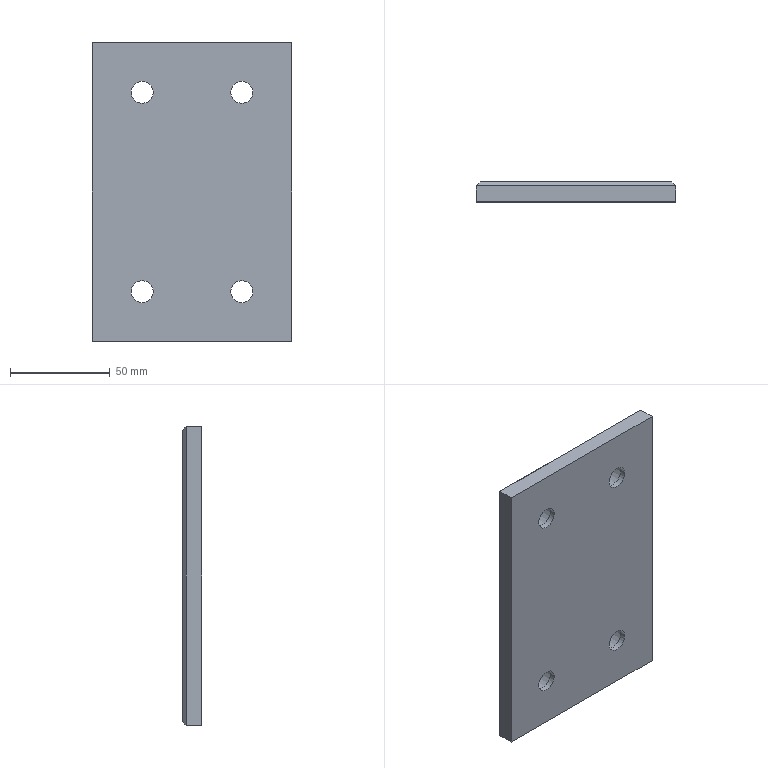Part | NX | features solid 2 | 1 solid | 22 faces | box 100 x 10 x 150 mm | volume 140961 mm3 | plane 14 | cylinder 8 | commonest cylinder face diameters 11 x4 17.5 x4
STEP:
#1=CARTESIAN_POINT('',(45.,37.,109.));
#2=VERTEX_POINT('',#1);
#3=CARTESIAN_POINT('',(45.,45.,109.));
#4=VERTEX_POINT('',#3);
#5=CARTESIAN_POINT('',(45.,37.,109.));
#6=DIRECTION('',(0.,1.,0.));
#7=VECTOR('',#6,1000.);
#8=LINE('',#5,#7);
#9=EDGE_CURVE('',#2,#4,#8,.T.);
#10=ORIENTED_EDGE('',*,*,#9,.T.);
#11=CARTESIAN_POINT('',(45.,45.,259.));
#12=VERTEX_POINT('',#11);
#13=CARTESIAN_POINT('',(45.,45.,259.));
#14=DIRECTION('',(0.,0.,1.));
#15=VECTOR('',#14,1000.);
#16=LINE('',#13,#15);
#17=EDGE_CURVE('',#4,#12,#16,.T.);
#18=ORIENTED_EDGE('',*,*,#17,.T.);
#19=CARTESIAN_POINT('',(45.,37.,259.));
#20=VERTEX_POINT('',#19);
#21=CARTESIAN_POINT('',(45.,37.,259.));
#22=DIRECTION('',(0.,1.,0.));
#23=VECTOR('',#22,1000.);
#24=LINE('',#21,#23);
#25=EDGE_CURVE('',#20,#12,#24,.T.);
#26=ORIENTED_EDGE('',*,*,#25,.F.);
#27=CARTESIAN_POINT('',(45.,37.,259.));
#28=DIRECTION('',(0.,0.,-1.));
#29=VECTOR('',#28,1000.);
#30=LINE('',#27,#29);
#31=EDGE_CURVE('',#2,#20,#30,.F.);
#32=ORIENTED_EDGE('',*,*,#31,.F.);
#33=EDGE_LOOP('',(#10,#18,#26,#32));
#34=FACE_BOUND('',#33,.T.);
#35=CARTESIAN_POINT('',(45.,37.,259.));
#36=DIRECTION('',(-1.,0.,0.));
#37=DIRECTION('',(0.,0.,1.));
#38=AXIS2_PLACEMENT_3D('',#35,#36,#37);
#39=PLANE('',#38);
#40=ADVANCED_FACE('',(#34),#39,.F.);
#41=CARTESIAN_POINT('',(-55.,37.,109.));
#42=VERTEX_POINT('',#41);
#43=CARTESIAN_POINT('',(-55.,45.,109.));
#44=VERTEX_POINT('',#43);
#45=CARTESIAN_POINT('',(-55.,37.,109.));
#46=DIRECTION('',(0.,1.,0.));
#47=VECTOR('',#46,1000.);
#48=LINE('',#45,#47);
#49=EDGE_CURVE('',#42,#44,#48,.T.);
#50=ORIENTED_EDGE('',*,*,#49,.T.);
#51=CARTESIAN_POINT('',(70.,45.,109.));
#52=DIRECTION('',(1.,0.,0.));
#53=VECTOR('',#52,1000.);
#54=LINE('',#51,#53);
#55=EDGE_CURVE('',#44,#4,#54,.T.);
#56=ORIENTED_EDGE('',*,*,#55,.T.);
#57=ORIENTED_EDGE('',*,*,#9,.F.);
#58=CARTESIAN_POINT('',(70.,37.,109.));
#59=DIRECTION('',(-1.,0.,0.));
#60=VECTOR('',#59,1000.);
#61=LINE('',#58,#60);
#62=EDGE_CURVE('',#2,#42,#61,.T.);
#63=ORIENTED_EDGE('',*,*,#62,.T.);
#64=EDGE_LOOP('',(#50,#56,#57,#63));
#65=FACE_BOUND('',#64,.T.);
#66=CARTESIAN_POINT('',(70.,37.,109.));
#67=DIRECTION('',(0.,0.,-1.));
#68=DIRECTION('',(-1.,0.,0.));
#69=AXIS2_PLACEMENT_3D('',#66,#67,#68);
#70=PLANE('',#69);
#71=ADVANCED_FACE('',(#65),#70,.T.);
#72=CARTESIAN_POINT('',(-55.,37.,259.));
#73=VERTEX_POINT('',#72);
#74=CARTESIAN_POINT('',(-55.,45.,259.));
#75=VERTEX_POINT('',#74);
#76=CARTESIAN_POINT('',(-55.,37.,259.));
#77=DIRECTION('',(0.,1.,0.));
#78=VECTOR('',#77,1000.);
#79=LINE('',#76,#78);
#80=EDGE_CURVE('',#73,#75,#79,.T.);
#81=ORIENTED_EDGE('',*,*,#80,.T.);
#82=CARTESIAN_POINT('',(-55.,45.,259.));
#83=DIRECTION('',(0.,0.,-1.));
#84=VECTOR('',#83,1000.);
#85=LINE('',#82,#84);
#86=EDGE_CURVE('',#75,#44,#85,.T.);
#87=ORIENTED_EDGE('',*,*,#86,.T.);
#88=ORIENTED_EDGE('',*,*,#49,.F.);
#89=CARTESIAN_POINT('',(-55.,37.,259.));
#90=DIRECTION('',(0.,0.,1.));
#91=VECTOR('',#90,1000.);
#92=LINE('',#89,#91);
#93=EDGE_CURVE('',#73,#42,#92,.F.);
#94=ORIENTED_EDGE('',*,*,#93,.F.);
#95=EDGE_LOOP('',(#81,#87,#88,#94));
#96=FACE_BOUND('',#95,.T.);
#97=CARTESIAN_POINT('',(-55.,37.,259.));
#98=DIRECTION('',(1.,0.,0.));
#99=DIRECTION('',(0.,0.,-1.));
#100=AXIS2_PLACEMENT_3D('',#97,#98,#99);
#101=PLANE('',#100);
#102=ADVANCED_FACE('',(#96),#101,.F.);
#103=ORIENTED_EDGE('',*,*,#25,.T.);
#104=CARTESIAN_POINT('',(-80.,45.,259.));
#105=DIRECTION('',(-1.,0.,0.));
#106=VECTOR('',#105,1000.);
#107=LINE('',#104,#106);
#108=EDGE_CURVE('',#12,#75,#107,.T.);
#109=ORIENTED_EDGE('',*,*,#108,.T.);
#110=ORIENTED_EDGE('',*,*,#80,.F.);
#111=CARTESIAN_POINT('',(-80.,37.,259.));
#112=DIRECTION('',(1.,0.,0.));
#113=VECTOR('',#112,1000.);
#114=LINE('',#111,#113);
#115=EDGE_CURVE('',#20,#73,#114,.F.);
#116=ORIENTED_EDGE('',*,*,#115,.F.);
#117=EDGE_LOOP('',(#103,#109,#110,#116));
#118=FACE_BOUND('',#117,.T.);
#119=CARTESIAN_POINT('',(-80.,37.,259.));
#120=DIRECTION('',(0.,0.,-1.));
#121=DIRECTION('',(-1.,0.,0.));
#122=AXIS2_PLACEMENT_3D('',#119,#120,#121);
#123=PLANE('',#122);
#124=ADVANCED_FACE('',(#118),#123,.F.);
#125=CARTESIAN_POINT('',(-30.,37.,228.5));
#126=VERTEX_POINT('',#125);
#127=CARTESIAN_POINT('',(-30.,37.,234.));
#128=DIRECTION('',(0.,-1.,0.));
#129=DIRECTION('',(0.,0.,-1.));
#130=AXIS2_PLACEMENT_3D('',#127,#128,#129);
#131=CIRCLE('',#130,5.5);
#132=EDGE_CURVE('',#126,#126,#131,.T.);
#133=ORIENTED_EDGE('',*,*,#132,.F.);
#134=EDGE_LOOP('',(#133));
#135=FACE_BOUND('',#134,.T.);
#136=CARTESIAN_POINT('',(20.,37.,228.5));
#137=VERTEX_POINT('',#136);
#138=CARTESIAN_POINT('',(20.,37.,234.));
#139=DIRECTION('',(0.,-1.,0.));
#140=DIRECTION('',(0.,0.,-1.));
#141=AXIS2_PLACEMENT_3D('',#138,#139,#140);
#142=CIRCLE('',#141,5.5);
#143=EDGE_CURVE('',#137,#137,#142,.T.);
#144=ORIENTED_EDGE('',*,*,#143,.F.);
#145=EDGE_LOOP('',(#144));
#146=FACE_BOUND('',#145,.T.);
#147=CARTESIAN_POINT('',(-30.,37.,128.5));
#148=VERTEX_POINT('',#147);
#149=CARTESIAN_POINT('',(-30.,37.,134.));
#150=DIRECTION('',(0.,-1.,0.));
#151=DIRECTION('',(0.,0.,-1.));
#152=AXIS2_PLACEMENT_3D('',#149,#150,#151);
#153=CIRCLE('',#152,5.5);
#154=EDGE_CURVE('',#148,#148,#153,.T.);
#155=ORIENTED_EDGE('',*,*,#154,.F.);
#156=EDGE_LOOP('',(#155));
#157=FACE_BOUND('',#156,.T.);
#158=CARTESIAN_POINT('',(20.,37.,128.5));
#159=VERTEX_POINT('',#158);
#160=CARTESIAN_POINT('',(20.,37.,134.));
#161=DIRECTION('',(0.,-1.,0.));
#162=DIRECTION('',(0.,0.,-1.));
#163=AXIS2_PLACEMENT_3D('',#160,#161,#162);
#164=CIRCLE('',#163,5.5);
#165=EDGE_CURVE('',#159,#159,#164,.T.);
#166=ORIENTED_EDGE('',*,*,#165,.F.);
#167=EDGE_LOOP('',(#166));
#168=FACE_BOUND('',#167,.T.);
#169=ORIENTED_EDGE('',*,*,#31,.T.);
#170=ORIENTED_EDGE('',*,*,#115,.T.);
#171=ORIENTED_EDGE('',*,*,#93,.T.);
#172=ORIENTED_EDGE('',*,*,#62,.F.);
#173=EDGE_LOOP('',(#169,#170,#171,#172));
#174=FACE_BOUND('',#173,.T.);
#175=CARTESIAN_POINT('',(70.,37.,259.));
#176=DIRECTION('',(0.,-1.,0.));
#177=DIRECTION('',(0.,0.,1.));
#178=AXIS2_PLACEMENT_3D('',#175,#176,#177);
#179=PLANE('',#178);
#180=ADVANCED_FACE('',(#135,#146,#157,#168,#174),#179,.T.);
#181=CARTESIAN_POINT('',(-30.,47.,225.25));
#182=VERTEX_POINT('',#181);
#183=CARTESIAN_POINT('',(-30.,47.,234.));
#184=DIRECTION('',(0.,-1.,0.));
#185=DIRECTION('',(0.,0.,-1.));
#186=AXIS2_PLACEMENT_3D('',#183,#184,#185);
#187=CIRCLE('',#186,8.75);
#188=EDGE_CURVE('',#182,#182,#187,.T.);
#189=ORIENTED_EDGE('',*,*,#188,.T.);
#190=EDGE_LOOP('',(#189));
#191=FACE_BOUND('',#190,.T.);
#192=CARTESIAN_POINT('',(20.,47.,225.25));
#193=VERTEX_POINT('',#192);
#194=CARTESIAN_POINT('',(20.,47.,234.));
#195=DIRECTION('',(0.,-1.,0.));
#196=DIRECTION('',(0.,0.,-1.));
#197=AXIS2_PLACEMENT_3D('',#194,#195,#196);
#198=CIRCLE('',#197,8.75);
#199=EDGE_CURVE('',#193,#193,#198,.T.);
#200=ORIENTED_EDGE('',*,*,#199,.T.);
#201=EDGE_LOOP('',(#200));
#202=FACE_BOUND('',#201,.T.);
#203=CARTESIAN_POINT('',(-30.,47.,125.25));
#204=VERTEX_POINT('',#203);
#205=CARTESIAN_POINT('',(-30.,47.,134.));
#206=DIRECTION('',(0.,-1.,0.));
#207=DIRECTION('',(0.,0.,-1.));
#208=AXIS2_PLACEMENT_3D('',#205,#206,#207);
#209=CIRCLE('',#208,8.75);
#210=EDGE_CURVE('',#204,#204,#209,.T.);
#211=ORIENTED_EDGE('',*,*,#210,.T.);
#212=EDGE_LOOP('',(#211));
#213=FACE_BOUND('',#212,.T.);
#214=CARTESIAN_POINT('',(20.,47.,125.25));
#215=VERTEX_POINT('',#214);
#216=CARTESIAN_POINT('',(20.,47.,134.));
#217=DIRECTION('',(0.,-1.,0.));
#218=DIRECTION('',(0.,0.,-1.));
#219=AXIS2_PLACEMENT_3D('',#216,#217,#218);
#220=CIRCLE('',#219,8.75);
#221=EDGE_CURVE('',#215,#215,#220,.T.);
#222=ORIENTED_EDGE('',*,*,#221,.T.);
#223=EDGE_LOOP('',(#222));
#224=FACE_BOUND('',#223,.T.);
#225=CARTESIAN_POINT('',(43.,47.,111.));
#226=VERTEX_POINT('',#225);
#227=CARTESIAN_POINT('',(-53.,47.,111.));
#228=VERTEX_POINT('',#227);
#229=CARTESIAN_POINT('',(-80.,47.,111.));
#230=DIRECTION('',(-1.,0.,0.));
#231=VECTOR('',#230,1000.);
#232=LINE('',#229,#231);
#233=EDGE_CURVE('',#226,#228,#232,.T.);
#234=ORIENTED_EDGE('',*,*,#233,.T.);
#235=CARTESIAN_POINT('',(-53.,47.,257.));
#236=VERTEX_POINT('',#235);
#237=CARTESIAN_POINT('',(-53.,47.,259.));
#238=DIRECTION('',(0.,0.,1.));
#239=VECTOR('',#238,1000.);
#240=LINE('',#237,#239);
#241=EDGE_CURVE('',#228,#236,#240,.T.);
#242=ORIENTED_EDGE('',*,*,#241,.T.);
#243=CARTESIAN_POINT('',(43.,47.,257.));
#244=VERTEX_POINT('',#243);
#245=CARTESIAN_POINT('',(70.,47.,257.));
#246=DIRECTION('',(1.,0.,0.));
#247=VECTOR('',#246,1000.);
#248=LINE('',#245,#247);
#249=EDGE_CURVE('',#236,#244,#248,.T.);
#250=ORIENTED_EDGE('',*,*,#249,.T.);
#251=CARTESIAN_POINT('',(43.,47.,259.));
#252=DIRECTION('',(0.,0.,-1.));
#253=VECTOR('',#252,1000.);
#254=LINE('',#251,#253);
#255=EDGE_CURVE('',#244,#226,#254,.T.);
#256=ORIENTED_EDGE('',*,*,#255,.T.);
#257=EDGE_LOOP('',(#234,#242,#250,#256));
#258=FACE_BOUND('',#257,.T.);
#259=CARTESIAN_POINT('',(70.,47.,259.));
#260=DIRECTION('',(0.,-1.,0.));
#261=DIRECTION('',(0.,0.,1.));
#262=AXIS2_PLACEMENT_3D('',#259,#260,#261);
#263=PLANE('',#262);
#264=ADVANCED_FACE('',(#191,#202,#213,#224,#258),#263,.F.);
#265=CARTESIAN_POINT('',(43.667,46.333,110.333));
#266=DIRECTION('',(-0.5774,0.5774,0.5774));
#267=VECTOR('',#266,1000.);
#268=LINE('',#265,#267);
#269=EDGE_CURVE('',#226,#4,#268,.F.);
#270=ORIENTED_EDGE('',*,*,#269,.F.);
#271=ORIENTED_EDGE('',*,*,#255,.F.);
#272=CARTESIAN_POINT('',(45.,45.,259.));
#273=DIRECTION('',(0.5774,-0.5774,0.5774));
#274=VECTOR('',#273,1000.);
#275=LINE('',#272,#274);
#276=EDGE_CURVE('',#12,#244,#275,.F.);
#277=ORIENTED_EDGE('',*,*,#276,.F.);
#278=ORIENTED_EDGE('',*,*,#17,.F.);
#279=EDGE_LOOP('',(#270,#271,#277,#278));
#280=FACE_BOUND('',#279,.T.);
#281=CARTESIAN_POINT('',(45.,45.,259.));
#282=DIRECTION('',(-0.7071,-0.7071,0.));
#283=DIRECTION('',(0.7071,-0.7071,0.));
#284=AXIS2_PLACEMENT_3D('',#281,#282,#283);
#285=PLANE('',#284);
#286=ADVANCED_FACE('',(#280),#285,.F.);
#287=ORIENTED_EDGE('',*,*,#276,.T.);
#288=ORIENTED_EDGE('',*,*,#249,.F.);
#289=CARTESIAN_POINT('',(-55.,45.,259.));
#290=DIRECTION('',(-0.5774,-0.5774,0.5774));
#291=VECTOR('',#290,1000.);
#292=LINE('',#289,#291);
#293=EDGE_CURVE('',#75,#236,#292,.F.);
#294=ORIENTED_EDGE('',*,*,#293,.F.);
#295=ORIENTED_EDGE('',*,*,#108,.F.);
#296=EDGE_LOOP('',(#287,#288,#294,#295));
#297=FACE_BOUND('',#296,.T.);
#298=CARTESIAN_POINT('',(-80.,45.,259.));
#299=DIRECTION('',(0.,-0.7071,-0.7071));
#300=DIRECTION('',(0.,0.7071,-0.7071));
#301=AXIS2_PLACEMENT_3D('',#298,#299,#300);
#302=PLANE('',#301);
#303=ADVANCED_FACE('',(#297),#302,.F.);
#304=ORIENTED_EDGE('',*,*,#269,.T.);
#305=ORIENTED_EDGE('',*,*,#55,.F.);
#306=CARTESIAN_POINT('',(-3.667,96.333,160.333));
#307=DIRECTION('',(-0.5774,-0.5774,-0.5774));
#308=VECTOR('',#307,1000.);
#309=LINE('',#306,#308);
#310=EDGE_CURVE('',#228,#44,#309,.T.);
#311=ORIENTED_EDGE('',*,*,#310,.F.);
#312=ORIENTED_EDGE('',*,*,#233,.F.);
#313=EDGE_LOOP('',(#304,#305,#311,#312));
#314=FACE_BOUND('',#313,.T.);
#315=CARTESIAN_POINT('',(70.,47.,111.));
#316=DIRECTION('',(0.,0.7071,-0.7071));
#317=DIRECTION('',(0.,0.7071,0.7071));
#318=AXIS2_PLACEMENT_3D('',#315,#316,#317);
#319=PLANE('',#318);
#320=ADVANCED_FACE('',(#314),#319,.T.);
#321=ORIENTED_EDGE('',*,*,#293,.T.);
#322=ORIENTED_EDGE('',*,*,#241,.F.);
#323=ORIENTED_EDGE('',*,*,#310,.T.);
#324=ORIENTED_EDGE('',*,*,#86,.F.);
#325=EDGE_LOOP('',(#321,#322,#323,#324));
#326=FACE_BOUND('',#325,.T.);
#327=CARTESIAN_POINT('',(-55.,45.,259.));
#328=DIRECTION('',(0.7071,-0.7071,0.));
#329=DIRECTION('',(0.7071,0.7071,0.));
#330=AXIS2_PLACEMENT_3D('',#327,#328,#329);
#331=PLANE('',#330);
#332=ADVANCED_FACE('',(#326),#331,.F.);
#333=ORIENTED_EDGE('',*,*,#165,.T.);
#334=EDGE_LOOP('',(#333));
#335=FACE_BOUND('',#334,.T.);
#336=CARTESIAN_POINT('',(20.,39.7,128.5));
#337=VERTEX_POINT('',#336);
#338=CARTESIAN_POINT('',(20.,39.7,134.));
#339=DIRECTION('',(0.,-1.,0.));
#340=DIRECTION('',(0.,0.,-1.));
#341=AXIS2_PLACEMENT_3D('',#338,#339,#340);
#342=CIRCLE('',#341,5.5);
#343=EDGE_CURVE('',#337,#337,#342,.T.);
#344=ORIENTED_EDGE('',*,*,#343,.F.);
#345=EDGE_LOOP('',(#344));
#346=FACE_BOUND('',#345,.T.);
#347=CARTESIAN_POINT('',(20.,-3.,134.));
#348=DIRECTION('',(0.,-1.,0.));
#349=DIRECTION('',(0.,0.,-1.));
#350=AXIS2_PLACEMENT_3D('',#347,#348,#349);
#351=CYLINDRICAL_SURFACE('',#350,5.5);
#352=ADVANCED_FACE('',(#335,#346),#351,.F.);
#353=ORIENTED_EDGE('',*,*,#343,.T.);
#354=EDGE_LOOP('',(#353));
#355=FACE_BOUND('',#354,.T.);
#356=CARTESIAN_POINT('',(20.,39.7,125.25));
#357=VERTEX_POINT('',#356);
#358=CARTESIAN_POINT('',(20.,39.7,134.));
#359=DIRECTION('',(0.,-1.,0.));
#360=DIRECTION('',(0.,0.,-1.));
#361=AXIS2_PLACEMENT_3D('',#358,#359,#360);
#362=CIRCLE('',#361,8.75);
#363=EDGE_CURVE('',#357,#357,#362,.T.);
#364=ORIENTED_EDGE('',*,*,#363,.F.);
#365=EDGE_LOOP('',(#364));
#366=FACE_BOUND('',#365,.T.);
#367=CARTESIAN_POINT('',(45.,39.7,134.));
#368=DIRECTION('',(0.,-1.,0.));
#369=DIRECTION('',(0.,0.,-1.));
#370=AXIS2_PLACEMENT_3D('',#367,#368,#369);
#371=PLANE('',#370);
#372=ADVANCED_FACE('',(#355,#366),#371,.F.);
#373=ORIENTED_EDGE('',*,*,#363,.T.);
#374=EDGE_LOOP('',(#373));
#375=FACE_BOUND('',#374,.T.);
#376=ORIENTED_EDGE('',*,*,#221,.F.);
#377=EDGE_LOOP('',(#376));
#378=FACE_BOUND('',#377,.T.);
#379=CARTESIAN_POINT('',(20.,47.,134.));
#380=DIRECTION('',(0.,-1.,0.));
#381=DIRECTION('',(0.,0.,-1.));
#382=AXIS2_PLACEMENT_3D('',#379,#380,#381);
#383=CYLINDRICAL_SURFACE('',#382,8.75);
#384=ADVANCED_FACE('',(#375,#378),#383,.F.);
#385=ORIENTED_EDGE('',*,*,#154,.T.);
#386=EDGE_LOOP('',(#385));
#387=FACE_BOUND('',#386,.T.);
#388=CARTESIAN_POINT('',(-30.,39.7,128.5));
#389=VERTEX_POINT('',#388);
#390=CARTESIAN_POINT('',(-30.,39.7,134.));
#391=DIRECTION('',(0.,-1.,0.));
#392=DIRECTION('',(0.,0.,-1.));
#393=AXIS2_PLACEMENT_3D('',#390,#391,#392);
#394=CIRCLE('',#393,5.5);
#395=EDGE_CURVE('',#389,#389,#394,.T.);
#396=ORIENTED_EDGE('',*,*,#395,.F.);
#397=EDGE_LOOP('',(#396));
#398=FACE_BOUND('',#397,.T.);
#399=CARTESIAN_POINT('',(-30.,-3.,134.));
#400=DIRECTION('',(0.,-1.,0.));
#401=DIRECTION('',(0.,0.,-1.));
#402=AXIS2_PLACEMENT_3D('',#399,#400,#401);
#403=CYLINDRICAL_SURFACE('',#402,5.5);
#404=ADVANCED_FACE('',(#387,#398),#403,.F.);
#405=ORIENTED_EDGE('',*,*,#395,.T.);
#406=EDGE_LOOP('',(#405));
#407=FACE_BOUND('',#406,.T.);
#408=CARTESIAN_POINT('',(-30.,39.7,125.25));
#409=VERTEX_POINT('',#408);
#410=CARTESIAN_POINT('',(-30.,39.7,134.));
#411=DIRECTION('',(0.,-1.,0.));
#412=DIRECTION('',(0.,0.,-1.));
#413=AXIS2_PLACEMENT_3D('',#410,#411,#412);
#414=CIRCLE('',#413,8.75);
#415=EDGE_CURVE('',#409,#409,#414,.T.);
#416=ORIENTED_EDGE('',*,*,#415,.F.);
#417=EDGE_LOOP('',(#416));
#418=FACE_BOUND('',#417,.T.);
#419=CARTESIAN_POINT('',(-55.,39.7,134.));
#420=DIRECTION('',(0.,-1.,0.));
#421=DIRECTION('',(0.,0.,-1.));
#422=AXIS2_PLACEMENT_3D('',#419,#420,#421);
#423=PLANE('',#422);
#424=ADVANCED_FACE('',(#407,#418),#423,.F.);
#425=ORIENTED_EDGE('',*,*,#415,.T.);
#426=EDGE_LOOP('',(#425));
#427=FACE_BOUND('',#426,.T.);
#428=ORIENTED_EDGE('',*,*,#210,.F.);
#429=EDGE_LOOP('',(#428));
#430=FACE_BOUND('',#429,.T.);
#431=CARTESIAN_POINT('',(-30.,47.,134.));
#432=DIRECTION('',(0.,-1.,0.));
#433=DIRECTION('',(0.,0.,-1.));
#434=AXIS2_PLACEMENT_3D('',#431,#432,#433);
#435=CYLINDRICAL_SURFACE('',#434,8.75);
#436=ADVANCED_FACE('',(#427,#430),#435,.F.);
#437=ORIENTED_EDGE('',*,*,#143,.T.);
#438=EDGE_LOOP('',(#437));
#439=FACE_BOUND('',#438,.T.);
#440=CARTESIAN_POINT('',(20.,39.7,228.5));
#441=VERTEX_POINT('',#440);
#442=CARTESIAN_POINT('',(20.,39.7,234.));
#443=DIRECTION('',(0.,-1.,0.));
#444=DIRECTION('',(0.,0.,-1.));
#445=AXIS2_PLACEMENT_3D('',#442,#443,#444);
#446=CIRCLE('',#445,5.5);
#447=EDGE_CURVE('',#441,#441,#446,.T.);
#448=ORIENTED_EDGE('',*,*,#447,.F.);
#449=EDGE_LOOP('',(#448));
#450=FACE_BOUND('',#449,.T.);
#451=CARTESIAN_POINT('',(20.,-3.,234.));
#452=DIRECTION('',(0.,-1.,0.));
#453=DIRECTION('',(0.,0.,-1.));
#454=AXIS2_PLACEMENT_3D('',#451,#452,#453);
#455=CYLINDRICAL_SURFACE('',#454,5.5);
#456=ADVANCED_FACE('',(#439,#450),#455,.F.);
#457=ORIENTED_EDGE('',*,*,#447,.T.);
#458=EDGE_LOOP('',(#457));
#459=FACE_BOUND('',#458,.T.);
#460=CARTESIAN_POINT('',(20.,39.7,225.25));
#461=VERTEX_POINT('',#460);
#462=CARTESIAN_POINT('',(20.,39.7,234.));
#463=DIRECTION('',(0.,-1.,0.));
#464=DIRECTION('',(0.,0.,-1.));
#465=AXIS2_PLACEMENT_3D('',#462,#463,#464);
#466=CIRCLE('',#465,8.75);
#467=EDGE_CURVE('',#461,#461,#466,.T.);
#468=ORIENTED_EDGE('',*,*,#467,.F.);
#469=EDGE_LOOP('',(#468));
#470=FACE_BOUND('',#469,.T.);
#471=CARTESIAN_POINT('',(45.,39.7,234.));
#472=DIRECTION('',(0.,-1.,0.));
#473=DIRECTION('',(0.,0.,-1.));
#474=AXIS2_PLACEMENT_3D('',#471,#472,#473);
#475=PLANE('',#474);
#476=ADVANCED_FACE('',(#459,#470),#475,.F.);
#477=ORIENTED_EDGE('',*,*,#467,.T.);
#478=EDGE_LOOP('',(#477));
#479=FACE_BOUND('',#478,.T.);
#480=ORIENTED_EDGE('',*,*,#199,.F.);
#481=EDGE_LOOP('',(#480));
#482=FACE_BOUND('',#481,.T.);
#483=CARTESIAN_POINT('',(20.,47.,234.));
#484=DIRECTION('',(0.,-1.,0.));
#485=DIRECTION('',(0.,0.,-1.));
#486=AXIS2_PLACEMENT_3D('',#483,#484,#485);
#487=CYLINDRICAL_SURFACE('',#486,8.75);
#488=ADVANCED_FACE('',(#479,#482),#487,.F.);
#489=ORIENTED_EDGE('',*,*,#132,.T.);
#490=EDGE_LOOP('',(#489));
#491=FACE_BOUND('',#490,.T.);
#492=CARTESIAN_POINT('',(-30.,39.7,228.5));
#493=VERTEX_POINT('',#492);
#494=CARTESIAN_POINT('',(-30.,39.7,234.));
#495=DIRECTION('',(0.,-1.,0.));
#496=DIRECTION('',(0.,0.,-1.));
#497=AXIS2_PLACEMENT_3D('',#494,#495,#496);
#498=CIRCLE('',#497,5.5);
#499=EDGE_CURVE('',#493,#493,#498,.T.);
#500=ORIENTED_EDGE('',*,*,#499,.F.);
#501=EDGE_LOOP('',(#500));
#502=FACE_BOUND('',#501,.T.);
#503=CARTESIAN_POINT('',(-30.,-3.,234.));
#504=DIRECTION('',(0.,-1.,0.));
#505=DIRECTION('',(0.,0.,-1.));
#506=AXIS2_PLACEMENT_3D('',#503,#504,#505);
#507=CYLINDRICAL_SURFACE('',#506,5.5);
#508=ADVANCED_FACE('',(#491,#502),#507,.F.);
#509=ORIENTED_EDGE('',*,*,#499,.T.);
#510=EDGE_LOOP('',(#509));
#511=FACE_BOUND('',#510,.T.);
#512=CARTESIAN_POINT('',(-30.,39.7,225.25));
#513=VERTEX_POINT('',#512);
#514=CARTESIAN_POINT('',(-30.,39.7,234.));
#515=DIRECTION('',(0.,-1.,0.));
#516=DIRECTION('',(0.,0.,-1.));
#517=AXIS2_PLACEMENT_3D('',#514,#515,#516);
#518=CIRCLE('',#517,8.75);
#519=EDGE_CURVE('',#513,#513,#518,.T.);
#520=ORIENTED_EDGE('',*,*,#519,.F.);
#521=EDGE_LOOP('',(#520));
#522=FACE_BOUND('',#521,.T.);
#523=CARTESIAN_POINT('',(-55.,39.7,234.));
#524=DIRECTION('',(0.,-1.,0.));
#525=DIRECTION('',(0.,0.,-1.));
#526=AXIS2_PLACEMENT_3D('',#523,#524,#525);
#527=PLANE('',#526);
#528=ADVANCED_FACE('',(#511,#522),#527,.F.);
#529=ORIENTED_EDGE('',*,*,#519,.T.);
#530=EDGE_LOOP('',(#529));
#531=FACE_BOUND('',#530,.T.);
#532=ORIENTED_EDGE('',*,*,#188,.F.);
#533=EDGE_LOOP('',(#532));
#534=FACE_BOUND('',#533,.T.);
#535=CARTESIAN_POINT('',(-30.,47.,234.));
#536=DIRECTION('',(0.,-1.,0.));
#537=DIRECTION('',(0.,0.,-1.));
#538=AXIS2_PLACEMENT_3D('',#535,#536,#537);
#539=CYLINDRICAL_SURFACE('',#538,8.75);
#540=ADVANCED_FACE('',(#531,#534),#539,.F.);
#541=CLOSED_SHELL('',(#40,#71,#102,#124,#180,#264,#286,#303,#320,#332,#352,#372,#384,#404,#424,#436,#456,#476,#488,#508,#528,#540));
#542=MANIFOLD_SOLID_BREP('',#541);
#543=(LENGTH_UNIT()NAMED_UNIT(*)SI_UNIT(.MILLI.,.METRE.));
#544=UNCERTAINTY_MEASURE_WITH_UNIT(LENGTH_MEASURE(0.00001),#543,'','');
#545=(NAMED_UNIT(*)PLANE_ANGLE_UNIT()SI_UNIT($,.RADIAN.));
#546=(NAMED_UNIT(*)SI_UNIT($,.STERADIAN.)SOLID_ANGLE_UNIT());
#547=(GEOMETRIC_REPRESENTATION_CONTEXT(3)GLOBAL_UNCERTAINTY_ASSIGNED_CONTEXT((#544))GLOBAL_UNIT_ASSIGNED_CONTEXT((#543,#545,#546))REPRESENTATION_CONTEXT('',''));
#548=ADVANCED_BREP_SHAPE_REPRESENTATION('',(#542),#547);